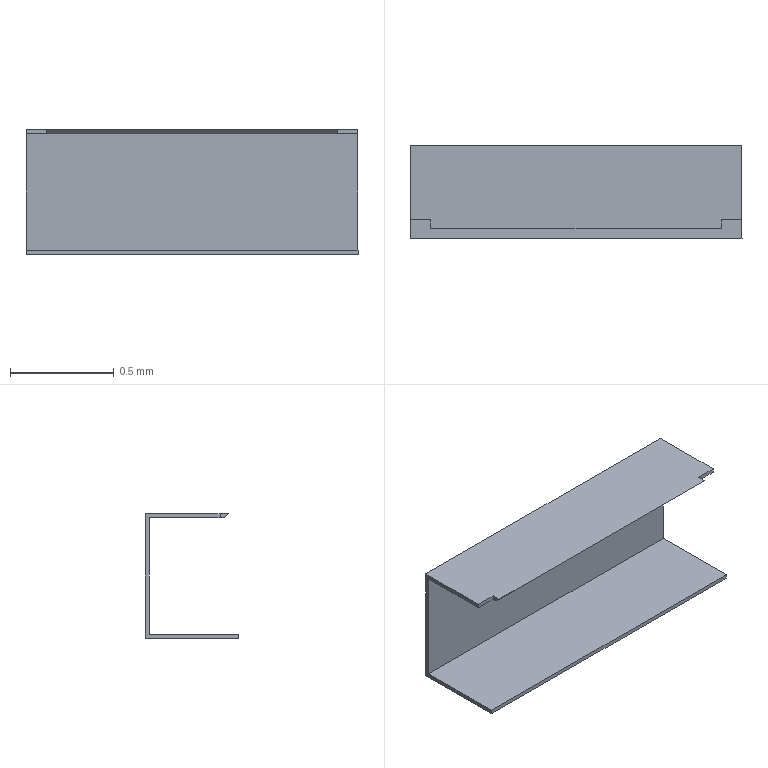Part | STEP file | RJ-USIO-V1_2-220411_11 | 1 solid | 14 faces | box 1.6 x 0.45 x 0.6 mm | volume 0.04468 mm3 | plane 14
STEP:
#1=CARTESIAN_POINT('',(0.,0.,0.));
#2=DIRECTION('',(0.,0.,1.));
#3=DIRECTION('',(1.,0.,0.));
#4=AXIS2_PLACEMENT_3D('',#1,#2,#3);
#5=CARTESIAN_POINT('',(52.5,20.72,0.58));
#6=VERTEX_POINT('',#5);
#7=CARTESIAN_POINT('',(52.5,20.74,0.58));
#8=VERTEX_POINT('',#7);
#9=CARTESIAN_POINT('',(52.5,20.72,0.58));
#10=DIRECTION('',(-0.000000044,1.,0.));
#11=VECTOR('',#10,1.);
#12=LINE('',#9,#11);
#13=CARTESIAN_POINT('',(52.5,20.74,-0.001));
#14=DIRECTION('',(-1.,-0.000000044,0.));
#15=DIRECTION('',(-0.000000044,1.,0.));
#16=AXIS2_PLACEMENT_3D('',#13,#14,#15);
#17=PLANE('',#16);
#18=CARTESIAN_POINT('',(-0.02,-0.581));
#19=DIRECTION('',(1.,0.));
#20=VECTOR('',#19,1.);
#21=LINE('',#18,#20);
#22=(GEOMETRIC_REPRESENTATION_CONTEXT(2)PARAMETRIC_REPRESENTATION_CONTEXT()REPRESENTATION_CONTEXT('',''));
#23=DEFINITIONAL_REPRESENTATION('',(#21),#22);
#24=PCURVE('',#17,#23);
#25=CARTESIAN_POINT('',(52.6,20.72,0.58));
#26=DIRECTION('',(0.,0.,-1.));
#27=DIRECTION('',(-0.000000044,1.,0.));
#28=AXIS2_PLACEMENT_3D('',#25,#26,#27);
#29=PLANE('',#28);
#30=CARTESIAN_POINT('',(0.,-0.1));
#31=DIRECTION('',(1.,0.));
#32=VECTOR('',#31,1.);
#33=LINE('',#30,#32);
#34=(GEOMETRIC_REPRESENTATION_CONTEXT(2)PARAMETRIC_REPRESENTATION_CONTEXT()REPRESENTATION_CONTEXT('',''));
#35=DEFINITIONAL_REPRESENTATION('',(#33),#34);
#36=PCURVE('',#29,#35);
#37=SURFACE_CURVE('',#12,(#24,#36),.PCURVE_S1.);
#38=EDGE_CURVE('',#6,#8,#37,.T.);
#39=ORIENTED_EDGE('',*,*,#38,.F.);
#40=CARTESIAN_POINT('',(52.5,20.7,0.6));
#41=VERTEX_POINT('',#40);
#42=CARTESIAN_POINT('',(52.5,20.7,0.6));
#43=DIRECTION('',(-0.000000031,0.7071,-0.7071));
#44=VECTOR('',#43,1.);
#45=LINE('',#42,#44);
#46=CARTESIAN_POINT('',(-0.04,-0.601));
#47=DIRECTION('',(0.7071,0.7071));
#48=VECTOR('',#47,1.);
#49=LINE('',#46,#48);
#50=(GEOMETRIC_REPRESENTATION_CONTEXT(2)PARAMETRIC_REPRESENTATION_CONTEXT()REPRESENTATION_CONTEXT('',''));
#51=DEFINITIONAL_REPRESENTATION('',(#49),#50);
#52=PCURVE('',#17,#51);
#53=CARTESIAN_POINT('',(52.6,20.7,0.6));
#54=DIRECTION('',(0.000000031,-0.7071,-0.7071));
#55=DIRECTION('',(-0.000000031,0.7071,-0.7071));
#56=AXIS2_PLACEMENT_3D('',#53,#54,#55);
#57=PLANE('',#56);
#58=CARTESIAN_POINT('',(0.,-0.1));
#59=DIRECTION('',(1.,0.));
#60=VECTOR('',#59,1.);
#61=LINE('',#58,#60);
#62=(GEOMETRIC_REPRESENTATION_CONTEXT(2)PARAMETRIC_REPRESENTATION_CONTEXT()REPRESENTATION_CONTEXT('',''));
#63=DEFINITIONAL_REPRESENTATION('',(#61),#62);
#64=PCURVE('',#57,#63);
#65=SURFACE_CURVE('',#45,(#52,#64),.PCURVE_S1.);
#66=EDGE_CURVE('',#41,#6,#65,.T.);
#67=ORIENTED_EDGE('',*,*,#66,.F.);
#68=CARTESIAN_POINT('',(52.5,20.74,0.6));
#69=VERTEX_POINT('',#68);
#70=CARTESIAN_POINT('',(52.5,20.7,0.6));
#71=DIRECTION('',(-0.000000044,1.,0.));
#72=VECTOR('',#71,1.);
#73=LINE('',#70,#72);
#74=CARTESIAN_POINT('',(-0.04,-0.601));
#75=DIRECTION('',(1.,0.));
#76=VECTOR('',#75,1.);
#77=LINE('',#74,#76);
#78=(GEOMETRIC_REPRESENTATION_CONTEXT(2)PARAMETRIC_REPRESENTATION_CONTEXT()REPRESENTATION_CONTEXT('',''));
#79=DEFINITIONAL_REPRESENTATION('',(#77),#78);
#80=PCURVE('',#17,#79);
#81=CARTESIAN_POINT('',(52.6,21.1,0.6));
#82=DIRECTION('',(0.,0.,1.));
#83=DIRECTION('',(0.000000044,-1.,0.));
#84=AXIS2_PLACEMENT_3D('',#81,#82,#83);
#85=PLANE('',#84);
#86=CARTESIAN_POINT('',(0.4,-0.1));
#87=DIRECTION('',(-1.,0.));
#88=VECTOR('',#87,1.);
#89=LINE('',#86,#88);
#90=(GEOMETRIC_REPRESENTATION_CONTEXT(2)PARAMETRIC_REPRESENTATION_CONTEXT()REPRESENTATION_CONTEXT('',''));
#91=DEFINITIONAL_REPRESENTATION('',(#89),#90);
#92=PCURVE('',#85,#91);
#93=SURFACE_CURVE('',#73,(#80,#92),.PCURVE_S1.);
#94=EDGE_CURVE('',#41,#69,#93,.T.);
#95=ORIENTED_EDGE('',*,*,#94,.T.);
#96=CARTESIAN_POINT('',(52.5,20.74,0.6));
#97=DIRECTION('',(0.,0.,-1.));
#98=VECTOR('',#97,1.);
#99=LINE('',#96,#98);
#100=CARTESIAN_POINT('',(0.,-0.601));
#101=DIRECTION('',(0.,1.));
#102=VECTOR('',#101,1.);
#103=LINE('',#100,#102);
#104=(GEOMETRIC_REPRESENTATION_CONTEXT(2)PARAMETRIC_REPRESENTATION_CONTEXT()REPRESENTATION_CONTEXT('',''));
#105=DEFINITIONAL_REPRESENTATION('',(#103),#104);
#106=PCURVE('',#17,#105);
#107=CARTESIAN_POINT('',(52.6,20.74,-0.001));
#108=DIRECTION('',(-0.000000044,1.,0.));
#109=DIRECTION('',(0.,0.,1.));
#110=AXIS2_PLACEMENT_3D('',#107,#108,#109);
#111=PLANE('',#110);
#112=CARTESIAN_POINT('',(0.601,-0.1));
#113=DIRECTION('',(-1.,0.));
#114=VECTOR('',#113,1.);
#115=LINE('',#112,#114);
#116=(GEOMETRIC_REPRESENTATION_CONTEXT(2)PARAMETRIC_REPRESENTATION_CONTEXT()REPRESENTATION_CONTEXT('',''));
#117=DEFINITIONAL_REPRESENTATION('',(#115),#116);
#118=PCURVE('',#111,#117);
#119=SURFACE_CURVE('',#99,(#106,#118),.PCURVE_S1.);
#120=EDGE_CURVE('',#69,#8,#119,.T.);
#121=ORIENTED_EDGE('',*,*,#120,.T.);
#122=EDGE_LOOP('',(#39,#67,#95,#121));
#123=FACE_BOUND('',#122,.F.);
#124=ADVANCED_FACE('',(#123),#17,.F.);
#125=CARTESIAN_POINT('',(51.1,20.74,0.58));
#126=VERTEX_POINT('',#125);
#127=CARTESIAN_POINT('',(51.1,20.72,0.58));
#128=VERTEX_POINT('',#127);
#129=CARTESIAN_POINT('',(51.1,20.74,0.58));
#130=DIRECTION('',(0.000000044,-1.,0.));
#131=VECTOR('',#130,1.);
#132=LINE('',#129,#131);
#133=CARTESIAN_POINT('',(0.02,-1.5));
#134=DIRECTION('',(-1.,0.));
#135=VECTOR('',#134,1.);
#136=LINE('',#133,#135);
#137=(GEOMETRIC_REPRESENTATION_CONTEXT(2)PARAMETRIC_REPRESENTATION_CONTEXT()REPRESENTATION_CONTEXT('',''));
#138=DEFINITIONAL_REPRESENTATION('',(#136),#137);
#139=PCURVE('',#29,#138);
#140=CARTESIAN_POINT('',(51.1,20.74,-0.001));
#141=DIRECTION('',(1.,0.000000044,0.));
#142=DIRECTION('',(0.000000044,-1.,0.));
#143=AXIS2_PLACEMENT_3D('',#140,#141,#142);
#144=PLANE('',#143);
#145=CARTESIAN_POINT('',(0.,-0.581));
#146=DIRECTION('',(1.,0.));
#147=VECTOR('',#146,1.);
#148=LINE('',#145,#147);
#149=(GEOMETRIC_REPRESENTATION_CONTEXT(2)PARAMETRIC_REPRESENTATION_CONTEXT()REPRESENTATION_CONTEXT('',''));
#150=DEFINITIONAL_REPRESENTATION('',(#148),#149);
#151=PCURVE('',#144,#150);
#152=SURFACE_CURVE('',#132,(#139,#151),.PCURVE_S1.);
#153=EDGE_CURVE('',#126,#128,#152,.T.);
#154=ORIENTED_EDGE('',*,*,#153,.T.);
#155=CARTESIAN_POINT('',(51.1,20.72,0.58));
#156=DIRECTION('',(1.,0.000000044,0.));
#157=VECTOR('',#156,1.);
#158=LINE('',#155,#157);
#159=CARTESIAN_POINT('',(0.,-1.5));
#160=DIRECTION('',(0.,1.));
#161=VECTOR('',#160,1.);
#162=LINE('',#159,#161);
#163=(GEOMETRIC_REPRESENTATION_CONTEXT(2)PARAMETRIC_REPRESENTATION_CONTEXT()REPRESENTATION_CONTEXT('',''));
#164=DEFINITIONAL_REPRESENTATION('',(#162),#163);
#165=PCURVE('',#29,#164);
#166=CARTESIAN_POINT('',(0.02828,-1.5));
#167=DIRECTION('',(0.,1.));
#168=VECTOR('',#167,1.);
#169=LINE('',#166,#168);
#170=(GEOMETRIC_REPRESENTATION_CONTEXT(2)PARAMETRIC_REPRESENTATION_CONTEXT()REPRESENTATION_CONTEXT('',''));
#171=DEFINITIONAL_REPRESENTATION('',(#169),#170);
#172=PCURVE('',#57,#171);
#173=SURFACE_CURVE('',#158,(#165,#172),.PCURVE_S1.);
#174=EDGE_CURVE('',#128,#6,#173,.T.);
#175=ORIENTED_EDGE('',*,*,#174,.T.);
#176=ORIENTED_EDGE('',*,*,#38,.T.);
#177=CARTESIAN_POINT('',(52.6,20.74,0.58));
#178=VERTEX_POINT('',#177);
#179=CARTESIAN_POINT('',(52.5,20.74,0.58));
#180=DIRECTION('',(1.,0.000000044,0.));
#181=VECTOR('',#180,1.);
#182=LINE('',#179,#181);
#183=CARTESIAN_POINT('',(0.02,-0.1));
#184=DIRECTION('',(0.,1.));
#185=VECTOR('',#184,1.);
#186=LINE('',#183,#185);
#187=(GEOMETRIC_REPRESENTATION_CONTEXT(2)PARAMETRIC_REPRESENTATION_CONTEXT()REPRESENTATION_CONTEXT('',''));
#188=DEFINITIONAL_REPRESENTATION('',(#186),#187);
#189=PCURVE('',#29,#188);
#190=CARTESIAN_POINT('',(0.581,-0.1));
#191=DIRECTION('',(0.,1.));
#192=VECTOR('',#191,1.);
#193=LINE('',#190,#192);
#194=(GEOMETRIC_REPRESENTATION_CONTEXT(2)PARAMETRIC_REPRESENTATION_CONTEXT()REPRESENTATION_CONTEXT('',''));
#195=DEFINITIONAL_REPRESENTATION('',(#193),#194);
#196=PCURVE('',#111,#195);
#197=SURFACE_CURVE('',#182,(#189,#196),.PCURVE_S1.);
#198=EDGE_CURVE('',#8,#178,#197,.T.);
#199=ORIENTED_EDGE('',*,*,#198,.T.);
#200=CARTESIAN_POINT('',(52.6,21.08,0.58));
#201=VERTEX_POINT('',#200);
#202=CARTESIAN_POINT('',(52.6,20.74,0.58));
#203=DIRECTION('',(-0.000000044,1.,0.));
#204=VECTOR('',#203,1.);
#205=LINE('',#202,#204);
#206=CARTESIAN_POINT('',(0.02,0.));
#207=DIRECTION('',(1.,0.));
#208=VECTOR('',#207,1.);
#209=LINE('',#206,#208);
#210=(GEOMETRIC_REPRESENTATION_CONTEXT(2)PARAMETRIC_REPRESENTATION_CONTEXT()REPRESENTATION_CONTEXT('',''));
#211=DEFINITIONAL_REPRESENTATION('',(#209),#210);
#212=PCURVE('',#29,#211);
#213=CARTESIAN_POINT('',(52.6,19.5,0.));
#214=DIRECTION('',(1.,0.000000044,0.));
#215=DIRECTION('',(0.,0.,1.));
#216=AXIS2_PLACEMENT_3D('',#213,#214,#215);
#217=PLANE('',#216);
#218=CARTESIAN_POINT('',(0.58,-1.24));
#219=DIRECTION('',(0.,-1.));
#220=VECTOR('',#219,1.);
#221=LINE('',#218,#220);
#222=(GEOMETRIC_REPRESENTATION_CONTEXT(2)PARAMETRIC_REPRESENTATION_CONTEXT()REPRESENTATION_CONTEXT('',''));
#223=DEFINITIONAL_REPRESENTATION('',(#221),#222);
#224=PCURVE('',#217,#223);
#225=SURFACE_CURVE('',#205,(#212,#224),.PCURVE_S1.);
#226=EDGE_CURVE('',#178,#201,#225,.T.);
#227=ORIENTED_EDGE('',*,*,#226,.T.);
#228=CARTESIAN_POINT('',(51.,21.08,0.58));
#229=VERTEX_POINT('',#228);
#230=CARTESIAN_POINT('',(51.,21.08,0.58));
#231=DIRECTION('',(1.,0.000000044,0.));
#232=VECTOR('',#231,1.);
#233=LINE('',#230,#232);
#234=CARTESIAN_POINT('',(0.36,-1.6));
#235=DIRECTION('',(0.,1.));
#236=VECTOR('',#235,1.);
#237=LINE('',#234,#236);
#238=(GEOMETRIC_REPRESENTATION_CONTEXT(2)PARAMETRIC_REPRESENTATION_CONTEXT()REPRESENTATION_CONTEXT('',''));
#239=DEFINITIONAL_REPRESENTATION('',(#237),#238);
#240=PCURVE('',#29,#239);
#241=CARTESIAN_POINT('',(52.6,21.08,0.58));
#242=DIRECTION('',(0.000000044,-1.,0.));
#243=DIRECTION('',(0.,0.,-1.));
#244=AXIS2_PLACEMENT_3D('',#241,#242,#243);
#245=PLANE('',#244);
#246=CARTESIAN_POINT('',(0.,-1.6));
#247=DIRECTION('',(0.,1.));
#248=VECTOR('',#247,1.);
#249=LINE('',#246,#248);
#250=(GEOMETRIC_REPRESENTATION_CONTEXT(2)PARAMETRIC_REPRESENTATION_CONTEXT()REPRESENTATION_CONTEXT('',''));
#251=DEFINITIONAL_REPRESENTATION('',(#249),#250);
#252=PCURVE('',#245,#251);
#253=SURFACE_CURVE('',#233,(#240,#252),.PCURVE_S1.);
#254=EDGE_CURVE('',#229,#201,#253,.T.);
#255=ORIENTED_EDGE('',*,*,#254,.F.);
#256=CARTESIAN_POINT('',(51.,20.74,0.58));
#257=VERTEX_POINT('',#256);
#258=CARTESIAN_POINT('',(51.,20.74,0.58));
#259=DIRECTION('',(-0.000000044,1.,0.));
#260=VECTOR('',#259,1.);
#261=LINE('',#258,#260);
#262=CARTESIAN_POINT('',(0.02,-1.6));
#263=DIRECTION('',(1.,0.));
#264=VECTOR('',#263,1.);
#265=LINE('',#262,#264);
#266=(GEOMETRIC_REPRESENTATION_CONTEXT(2)PARAMETRIC_REPRESENTATION_CONTEXT()REPRESENTATION_CONTEXT('',''));
#267=DEFINITIONAL_REPRESENTATION('',(#265),#266);
#268=PCURVE('',#29,#267);
#269=CARTESIAN_POINT('',(51.,19.5,0.));
#270=DIRECTION('',(1.,0.000000044,0.));
#271=DIRECTION('',(0.,0.,1.));
#272=AXIS2_PLACEMENT_3D('',#269,#270,#271);
#273=PLANE('',#272);
#274=CARTESIAN_POINT('',(0.58,-1.24));
#275=DIRECTION('',(0.,-1.));
#276=VECTOR('',#275,1.);
#277=LINE('',#274,#276);
#278=(GEOMETRIC_REPRESENTATION_CONTEXT(2)PARAMETRIC_REPRESENTATION_CONTEXT()REPRESENTATION_CONTEXT('',''));
#279=DEFINITIONAL_REPRESENTATION('',(#277),#278);
#280=PCURVE('',#273,#279);
#281=SURFACE_CURVE('',#261,(#268,#280),.PCURVE_S1.);
#282=EDGE_CURVE('',#257,#229,#281,.T.);
#283=ORIENTED_EDGE('',*,*,#282,.F.);
#284=CARTESIAN_POINT('',(51.,20.74,0.58));
#285=DIRECTION('',(1.,0.000000044,0.));
#286=VECTOR('',#285,1.);
#287=LINE('',#284,#286);
#288=CARTESIAN_POINT('',(0.02,-1.6));
#289=DIRECTION('',(0.,1.));
#290=VECTOR('',#289,1.);
#291=LINE('',#288,#290);
#292=(GEOMETRIC_REPRESENTATION_CONTEXT(2)PARAMETRIC_REPRESENTATION_CONTEXT()REPRESENTATION_CONTEXT('',''));
#293=DEFINITIONAL_REPRESENTATION('',(#291),#292);
#294=PCURVE('',#29,#293);
#295=CARTESIAN_POINT('',(51.,20.74,-0.001));
#296=DIRECTION('',(-0.000000044,1.,0.));
#297=DIRECTION('',(0.,0.,1.));
#298=AXIS2_PLACEMENT_3D('',#295,#296,#297);
#299=PLANE('',#298);
#300=CARTESIAN_POINT('',(0.581,0.));
#301=DIRECTION('',(0.,1.));
#302=VECTOR('',#301,1.);
#303=LINE('',#300,#302);
#304=(GEOMETRIC_REPRESENTATION_CONTEXT(2)PARAMETRIC_REPRESENTATION_CONTEXT()REPRESENTATION_CONTEXT('',''));
#305=DEFINITIONAL_REPRESENTATION('',(#303),#304);
#306=PCURVE('',#299,#305);
#307=SURFACE_CURVE('',#287,(#294,#306),.PCURVE_S1.);
#308=EDGE_CURVE('',#257,#126,#307,.T.);
#309=ORIENTED_EDGE('',*,*,#308,.T.);
#310=EDGE_LOOP('',(#154,#175,#176,#199,#227,#255,#283,#309));
#311=FACE_BOUND('',#310,.F.);
#312=ADVANCED_FACE('',(#311),#29,.T.);
#313=CARTESIAN_POINT('',(51.1,20.74,0.6));
#314=VERTEX_POINT('',#313);
#315=CARTESIAN_POINT('',(51.1,20.7,0.6));
#316=VERTEX_POINT('',#315);
#317=CARTESIAN_POINT('',(51.1,20.74,0.6));
#318=DIRECTION('',(0.000000044,-1.,0.));
#319=VECTOR('',#318,1.);
#320=LINE('',#317,#319);
#321=CARTESIAN_POINT('',(0.,-0.601));
#322=DIRECTION('',(1.,0.));
#323=VECTOR('',#322,1.);
#324=LINE('',#321,#323);
#325=(GEOMETRIC_REPRESENTATION_CONTEXT(2)PARAMETRIC_REPRESENTATION_CONTEXT()REPRESENTATION_CONTEXT('',''));
#326=DEFINITIONAL_REPRESENTATION('',(#324),#325);
#327=PCURVE('',#144,#326);
#328=CARTESIAN_POINT('',(0.36,-1.5));
#329=DIRECTION('',(1.,0.));
#330=VECTOR('',#329,1.);
#331=LINE('',#328,#330);
#332=(GEOMETRIC_REPRESENTATION_CONTEXT(2)PARAMETRIC_REPRESENTATION_CONTEXT()REPRESENTATION_CONTEXT('',''));
#333=DEFINITIONAL_REPRESENTATION('',(#331),#332);
#334=PCURVE('',#85,#333);
#335=SURFACE_CURVE('',#320,(#327,#334),.PCURVE_S1.);
#336=EDGE_CURVE('',#314,#316,#335,.T.);
#337=ORIENTED_EDGE('',*,*,#336,.T.);
#338=CARTESIAN_POINT('',(51.1,20.72,0.58));
#339=DIRECTION('',(0.000000031,-0.7071,0.7071));
#340=VECTOR('',#339,1.);
#341=LINE('',#338,#340);
#342=CARTESIAN_POINT('',(0.02,-0.581));
#343=DIRECTION('',(0.7071,-0.7071));
#344=VECTOR('',#343,1.);
#345=LINE('',#342,#344);
#346=(GEOMETRIC_REPRESENTATION_CONTEXT(2)PARAMETRIC_REPRESENTATION_CONTEXT()REPRESENTATION_CONTEXT('',''));
#347=DEFINITIONAL_REPRESENTATION('',(#345),#346);
#348=PCURVE('',#144,#347);
#349=CARTESIAN_POINT('',(0.02828,-1.5));
#350=DIRECTION('',(-1.,0.));
#351=VECTOR('',#350,1.);
#352=LINE('',#349,#351);
#353=(GEOMETRIC_REPRESENTATION_CONTEXT(2)PARAMETRIC_REPRESENTATION_CONTEXT()REPRESENTATION_CONTEXT('',''));
#354=DEFINITIONAL_REPRESENTATION('',(#352),#353);
#355=PCURVE('',#57,#354);
#356=SURFACE_CURVE('',#341,(#348,#355),.PCURVE_S1.);
#357=EDGE_CURVE('',#128,#316,#356,.T.);
#358=ORIENTED_EDGE('',*,*,#357,.F.);
#359=ORIENTED_EDGE('',*,*,#153,.F.);
#360=CARTESIAN_POINT('',(51.1,20.74,0.6));
#361=DIRECTION('',(0.,0.,-1.));
#362=VECTOR('',#361,1.);
#363=LINE('',#360,#362);
#364=CARTESIAN_POINT('',(0.,-0.601));
#365=DIRECTION('',(0.,1.));
#366=VECTOR('',#365,1.);
#367=LINE('',#364,#366);
#368=(GEOMETRIC_REPRESENTATION_CONTEXT(2)PARAMETRIC_REPRESENTATION_CONTEXT()REPRESENTATION_CONTEXT('',''));
#369=DEFINITIONAL_REPRESENTATION('',(#367),#368);
#370=PCURVE('',#144,#369);
#371=CARTESIAN_POINT('',(0.601,0.1));
#372=DIRECTION('',(-1.,0.));
#373=VECTOR('',#372,1.);
#374=LINE('',#371,#373);
#375=(GEOMETRIC_REPRESENTATION_CONTEXT(2)PARAMETRIC_REPRESENTATION_CONTEXT()REPRESENTATION_CONTEXT('',''));
#376=DEFINITIONAL_REPRESENTATION('',(#374),#375);
#377=PCURVE('',#299,#376);
#378=SURFACE_CURVE('',#363,(#370,#377),.PCURVE_S1.);
#379=EDGE_CURVE('',#314,#126,#378,.T.);
#380=ORIENTED_EDGE('',*,*,#379,.F.);
#381=EDGE_LOOP('',(#337,#358,#359,#380));
#382=FACE_BOUND('',#381,.F.);
#383=ADVANCED_FACE('',(#382),#144,.F.);
#384=ORIENTED_EDGE('',*,*,#336,.F.);
#385=CARTESIAN_POINT('',(51.,20.74,0.6));
#386=VERTEX_POINT('',#385);
#387=CARTESIAN_POINT('',(51.,20.74,0.6));
#388=DIRECTION('',(1.,0.000000044,0.));
#389=VECTOR('',#388,1.);
#390=LINE('',#387,#389);
#391=CARTESIAN_POINT('',(0.36,-1.6));
#392=DIRECTION('',(0.,1.));
#393=VECTOR('',#392,1.);
#394=LINE('',#391,#393);
#395=(GEOMETRIC_REPRESENTATION_CONTEXT(2)PARAMETRIC_REPRESENTATION_CONTEXT()REPRESENTATION_CONTEXT('',''));
#396=DEFINITIONAL_REPRESENTATION('',(#394),#395);
#397=PCURVE('',#85,#396);
#398=CARTESIAN_POINT('',(0.601,0.));
#399=DIRECTION('',(0.,1.));
#400=VECTOR('',#399,1.);
#401=LINE('',#398,#400);
#402=(GEOMETRIC_REPRESENTATION_CONTEXT(2)PARAMETRIC_REPRESENTATION_CONTEXT()REPRESENTATION_CONTEXT('',''));
#403=DEFINITIONAL_REPRESENTATION('',(#401),#402);
#404=PCURVE('',#299,#403);
#405=SURFACE_CURVE('',#390,(#397,#404),.PCURVE_S1.);
#406=EDGE_CURVE('',#386,#314,#405,.T.);
#407=ORIENTED_EDGE('',*,*,#406,.F.);
#408=CARTESIAN_POINT('',(51.,21.1,0.6));
#409=VERTEX_POINT('',#408);
#410=CARTESIAN_POINT('',(51.,21.1,0.6));
#411=DIRECTION('',(0.000000044,-1.,0.));
#412=VECTOR('',#411,1.);
#413=LINE('',#410,#412);
#414=CARTESIAN_POINT('',(0.,-1.6));
#415=DIRECTION('',(1.,0.));
#416=VECTOR('',#415,1.);
#417=LINE('',#414,#416);
#418=(GEOMETRIC_REPRESENTATION_CONTEXT(2)PARAMETRIC_REPRESENTATION_CONTEXT()REPRESENTATION_CONTEXT('',''));
#419=DEFINITIONAL_REPRESENTATION('',(#417),#418);
#420=PCURVE('',#85,#419);
#421=CARTESIAN_POINT('',(0.6,-1.6));
#422=DIRECTION('',(0.,1.));
#423=VECTOR('',#422,1.);
#424=LINE('',#421,#423);
#425=(GEOMETRIC_REPRESENTATION_CONTEXT(2)PARAMETRIC_REPRESENTATION_CONTEXT()REPRESENTATION_CONTEXT('',''));
#426=DEFINITIONAL_REPRESENTATION('',(#424),#425);
#427=PCURVE('',#273,#426);
#428=SURFACE_CURVE('',#413,(#420,#427),.PCURVE_S1.);
#429=EDGE_CURVE('',#409,#386,#428,.T.);
#430=ORIENTED_EDGE('',*,*,#429,.F.);
#431=CARTESIAN_POINT('',(52.6,21.1,0.6));
#432=VERTEX_POINT('',#431);
#433=CARTESIAN_POINT('',(51.,21.1,0.6));
#434=DIRECTION('',(1.,0.000000044,0.));
#435=VECTOR('',#434,1.);
#436=LINE('',#433,#435);
#437=CARTESIAN_POINT('',(0.,-1.6));
#438=DIRECTION('',(0.,1.));
#439=VECTOR('',#438,1.);
#440=LINE('',#437,#439);
#441=(GEOMETRIC_REPRESENTATION_CONTEXT(2)PARAMETRIC_REPRESENTATION_CONTEXT()REPRESENTATION_CONTEXT('',''));
#442=DEFINITIONAL_REPRESENTATION('',(#440),#441);
#443=PCURVE('',#85,#442);
#444=CARTESIAN_POINT('',(52.6,21.1,0.));
#445=DIRECTION('',(-0.000000044,1.,0.));
#446=DIRECTION('',(0.,0.,1.));
#447=AXIS2_PLACEMENT_3D('',#444,#445,#446);
#448=PLANE('',#447);
#449=CARTESIAN_POINT('',(0.6,-1.6));
#450=DIRECTION('',(0.,1.));
#451=VECTOR('',#450,1.);
#452=LINE('',#449,#451);
#453=(GEOMETRIC_REPRESENTATION_CONTEXT(2)PARAMETRIC_REPRESENTATION_CONTEXT()REPRESENTATION_CONTEXT('',''));
#454=DEFINITIONAL_REPRESENTATION('',(#452),#453);
#455=PCURVE('',#448,#454);
#456=SURFACE_CURVE('',#436,(#443,#455),.PCURVE_S1.);
#457=EDGE_CURVE('',#409,#432,#456,.T.);
#458=ORIENTED_EDGE('',*,*,#457,.T.);
#459=CARTESIAN_POINT('',(52.6,20.74,0.6));
#460=VERTEX_POINT('',#459);
#461=CARTESIAN_POINT('',(52.6,21.1,0.6));
#462=DIRECTION('',(0.000000044,-1.,0.));
#463=VECTOR('',#462,1.);
#464=LINE('',#461,#463);
#465=CARTESIAN_POINT('',(0.,0.));
#466=DIRECTION('',(1.,0.));
#467=VECTOR('',#466,1.);
#468=LINE('',#465,#467);
#469=(GEOMETRIC_REPRESENTATION_CONTEXT(2)PARAMETRIC_REPRESENTATION_CONTEXT()REPRESENTATION_CONTEXT('',''));
#470=DEFINITIONAL_REPRESENTATION('',(#468),#469);
#471=PCURVE('',#85,#470);
#472=CARTESIAN_POINT('',(0.6,-1.6));
#473=DIRECTION('',(0.,1.));
#474=VECTOR('',#473,1.);
#475=LINE('',#472,#474);
#476=(GEOMETRIC_REPRESENTATION_CONTEXT(2)PARAMETRIC_REPRESENTATION_CONTEXT()REPRESENTATION_CONTEXT('',''));
#477=DEFINITIONAL_REPRESENTATION('',(#475),#476);
#478=PCURVE('',#217,#477);
#479=SURFACE_CURVE('',#464,(#471,#478),.PCURVE_S1.);
#480=EDGE_CURVE('',#432,#460,#479,.T.);
#481=ORIENTED_EDGE('',*,*,#480,.T.);
#482=CARTESIAN_POINT('',(52.5,20.74,0.6));
#483=DIRECTION('',(1.,0.000000044,0.));
#484=VECTOR('',#483,1.);
#485=LINE('',#482,#484);
#486=CARTESIAN_POINT('',(0.36,-0.1));
#487=DIRECTION('',(0.,1.));
#488=VECTOR('',#487,1.);
#489=LINE('',#486,#488);
#490=(GEOMETRIC_REPRESENTATION_CONTEXT(2)PARAMETRIC_REPRESENTATION_CONTEXT()REPRESENTATION_CONTEXT('',''));
#491=DEFINITIONAL_REPRESENTATION('',(#489),#490);
#492=PCURVE('',#85,#491);
#493=CARTESIAN_POINT('',(0.601,-0.1));
#494=DIRECTION('',(0.,1.));
#495=VECTOR('',#494,1.);
#496=LINE('',#493,#495);
#497=(GEOMETRIC_REPRESENTATION_CONTEXT(2)PARAMETRIC_REPRESENTATION_CONTEXT()REPRESENTATION_CONTEXT('',''));
#498=DEFINITIONAL_REPRESENTATION('',(#496),#497);
#499=PCURVE('',#111,#498);
#500=SURFACE_CURVE('',#485,(#492,#499),.PCURVE_S1.);
#501=EDGE_CURVE('',#69,#460,#500,.T.);
#502=ORIENTED_EDGE('',*,*,#501,.F.);
#503=ORIENTED_EDGE('',*,*,#94,.F.);
#504=CARTESIAN_POINT('',(51.1,20.7,0.6));
#505=DIRECTION('',(1.,0.000000044,0.));
#506=VECTOR('',#505,1.);
#507=LINE('',#504,#506);
#508=CARTESIAN_POINT('',(0.4,-1.5));
#509=DIRECTION('',(0.,1.));
#510=VECTOR('',#509,1.);
#511=LINE('',#508,#510);
#512=(GEOMETRIC_REPRESENTATION_CONTEXT(2)PARAMETRIC_REPRESENTATION_CONTEXT()REPRESENTATION_CONTEXT('',''));
#513=DEFINITIONAL_REPRESENTATION('',(#511),#512);
#514=PCURVE('',#85,#513);
#515=CARTESIAN_POINT('',(0.,-1.5));
#516=DIRECTION('',(0.,1.));
#517=VECTOR('',#516,1.);
#518=LINE('',#515,#517);
#519=(GEOMETRIC_REPRESENTATION_CONTEXT(2)PARAMETRIC_REPRESENTATION_CONTEXT()REPRESENTATION_CONTEXT('',''));
#520=DEFINITIONAL_REPRESENTATION('',(#518),#519);
#521=PCURVE('',#57,#520);
#522=SURFACE_CURVE('',#507,(#514,#521),.PCURVE_S1.);
#523=EDGE_CURVE('',#316,#41,#522,.T.);
#524=ORIENTED_EDGE('',*,*,#523,.F.);
#525=EDGE_LOOP('',(#384,#407,#430,#458,#481,#502,#503,#524));
#526=FACE_BOUND('',#525,.F.);
#527=ADVANCED_FACE('',(#526),#85,.T.);
#528=ORIENTED_EDGE('',*,*,#379,.T.);
#529=ORIENTED_EDGE('',*,*,#308,.F.);
#530=CARTESIAN_POINT('',(51.,20.74,0.6));
#531=DIRECTION('',(0.,0.,-1.));
#532=VECTOR('',#531,1.);
#533=LINE('',#530,#532);
#534=CARTESIAN_POINT('',(0.601,0.));
#535=DIRECTION('',(-1.,0.));
#536=VECTOR('',#535,1.);
#537=LINE('',#534,#536);
#538=(GEOMETRIC_REPRESENTATION_CONTEXT(2)PARAMETRIC_REPRESENTATION_CONTEXT()REPRESENTATION_CONTEXT('',''));
#539=DEFINITIONAL_REPRESENTATION('',(#537),#538);
#540=PCURVE('',#299,#539);
#541=CARTESIAN_POINT('',(0.6,-1.24));
#542=DIRECTION('',(-1.,0.));
#543=VECTOR('',#542,1.);
#544=LINE('',#541,#543);
#545=(GEOMETRIC_REPRESENTATION_CONTEXT(2)PARAMETRIC_REPRESENTATION_CONTEXT()REPRESENTATION_CONTEXT('',''));
#546=DEFINITIONAL_REPRESENTATION('',(#544),#545);
#547=PCURVE('',#273,#546);
#548=SURFACE_CURVE('',#533,(#540,#547),.PCURVE_S1.);
#549=EDGE_CURVE('',#386,#257,#548,.T.);
#550=ORIENTED_EDGE('',*,*,#549,.F.);
#551=ORIENTED_EDGE('',*,*,#406,.T.);
#552=EDGE_LOOP('',(#528,#529,#550,#551));
#553=FACE_BOUND('',#552,.F.);
#554=ADVANCED_FACE('',(#553),#299,.F.);
#555=ORIENTED_EDGE('',*,*,#282,.T.);
#556=CARTESIAN_POINT('',(51.,21.08,0.02));
#557=VERTEX_POINT('',#556);
#558=CARTESIAN_POINT('',(51.,21.08,0.58));
#559=DIRECTION('',(0.,0.,-1.));
#560=VECTOR('',#559,1.);
#561=LINE('',#558,#560);
#562=CARTESIAN_POINT('',(0.58,-1.58));
#563=DIRECTION('',(-1.,0.));
#564=VECTOR('',#563,1.);
#565=LINE('',#562,#564);
#566=(GEOMETRIC_REPRESENTATION_CONTEXT(2)PARAMETRIC_REPRESENTATION_CONTEXT()REPRESENTATION_CONTEXT('',''));
#567=DEFINITIONAL_REPRESENTATION('',(#565),#566);
#568=PCURVE('',#273,#567);
#569=CARTESIAN_POINT('',(0.,-1.6));
#570=DIRECTION('',(1.,0.));
#571=VECTOR('',#570,1.);
#572=LINE('',#569,#571);
#573=(GEOMETRIC_REPRESENTATION_CONTEXT(2)PARAMETRIC_REPRESENTATION_CONTEXT()REPRESENTATION_CONTEXT('',''));
#574=DEFINITIONAL_REPRESENTATION('',(#572),#573);
#575=PCURVE('',#245,#574);
#576=SURFACE_CURVE('',#561,(#568,#575),.PCURVE_S1.);
#577=EDGE_CURVE('',#229,#557,#576,.T.);
#578=ORIENTED_EDGE('',*,*,#577,.T.);
#579=CARTESIAN_POINT('',(51.,20.65,0.02));
#580=VERTEX_POINT('',#579);
#581=CARTESIAN_POINT('',(51.,21.08,0.02));
#582=DIRECTION('',(0.000000044,-1.,0.));
#583=VECTOR('',#582,1.);
#584=LINE('',#581,#583);
#585=CARTESIAN_POINT('',(0.02,-1.58));
#586=DIRECTION('',(0.,1.));
#587=VECTOR('',#586,1.);
#588=LINE('',#585,#587);
#589=(GEOMETRIC_REPRESENTATION_CONTEXT(2)PARAMETRIC_REPRESENTATION_CONTEXT()REPRESENTATION_CONTEXT('',''));
#590=DEFINITIONAL_REPRESENTATION('',(#588),#589);
#591=PCURVE('',#273,#590);
#592=CARTESIAN_POINT('',(52.6,21.08,0.02));
#593=DIRECTION('',(0.,0.,1.));
#594=DIRECTION('',(0.000000044,-1.,0.));
#595=AXIS2_PLACEMENT_3D('',#592,#593,#594);
#596=PLANE('',#595);
#597=CARTESIAN_POINT('',(0.,-1.6));
#598=DIRECTION('',(1.,0.));
#599=VECTOR('',#598,1.);
#600=LINE('',#597,#599);
#601=(GEOMETRIC_REPRESENTATION_CONTEXT(2)PARAMETRIC_REPRESENTATION_CONTEXT()REPRESENTATION_CONTEXT('',''));
#602=DEFINITIONAL_REPRESENTATION('',(#600),#601);
#603=PCURVE('',#596,#602);
#604=SURFACE_CURVE('',#584,(#591,#603),.PCURVE_S1.);
#605=EDGE_CURVE('',#557,#580,#604,.T.);
#606=ORIENTED_EDGE('',*,*,#605,.T.);
#607=CARTESIAN_POINT('',(51.,20.65,0.));
#608=VERTEX_POINT('',#607);
#609=CARTESIAN_POINT('',(51.,20.65,0.02));
#610=DIRECTION('',(0.,0.,-1.));
#611=VECTOR('',#610,1.);
#612=LINE('',#609,#611);
#613=CARTESIAN_POINT('',(0.02,-1.15));
#614=DIRECTION('',(-1.,0.));
#615=VECTOR('',#614,1.);
#616=LINE('',#613,#615);
#617=(GEOMETRIC_REPRESENTATION_CONTEXT(2)PARAMETRIC_REPRESENTATION_CONTEXT()REPRESENTATION_CONTEXT('',''));
#618=DEFINITIONAL_REPRESENTATION('',(#616),#617);
#619=PCURVE('',#273,#618);
#620=CARTESIAN_POINT('',(52.6,20.65,0.02));
#621=DIRECTION('',(0.000000044,-1.,0.));
#622=DIRECTION('',(0.,0.,-1.));
#623=AXIS2_PLACEMENT_3D('',#620,#621,#622);
#624=PLANE('',#623);
#625=CARTESIAN_POINT('',(0.,-1.6));
#626=DIRECTION('',(1.,0.));
#627=VECTOR('',#626,1.);
#628=LINE('',#625,#627);
#629=(GEOMETRIC_REPRESENTATION_CONTEXT(2)PARAMETRIC_REPRESENTATION_CONTEXT()REPRESENTATION_CONTEXT('',''));
#630=DEFINITIONAL_REPRESENTATION('',(#628),#629);
#631=PCURVE('',#624,#630);
#632=SURFACE_CURVE('',#612,(#619,#631),.PCURVE_S1.);
#633=EDGE_CURVE('',#580,#608,#632,.T.);
#634=ORIENTED_EDGE('',*,*,#633,.T.);
#635=CARTESIAN_POINT('',(51.,21.1,0.));
#636=VERTEX_POINT('',#635);
#637=CARTESIAN_POINT('',(51.,20.65,0.));
#638=DIRECTION('',(-0.000000044,1.,0.));
#639=VECTOR('',#638,1.);
#640=LINE('',#637,#639);
#641=CARTESIAN_POINT('',(0.,-1.15));
#642=DIRECTION('',(0.,-1.));
#643=VECTOR('',#642,1.);
#644=LINE('',#641,#643);
#645=(GEOMETRIC_REPRESENTATION_CONTEXT(2)PARAMETRIC_REPRESENTATION_CONTEXT()REPRESENTATION_CONTEXT('',''));
#646=DEFINITIONAL_REPRESENTATION('',(#644),#645);
#647=PCURVE('',#273,#646);
#648=CARTESIAN_POINT('',(52.6,20.65,0.));
#649=DIRECTION('',(0.,0.,-1.));
#650=DIRECTION('',(-0.000000044,1.,0.));
#651=AXIS2_PLACEMENT_3D('',#648,#649,#650);
#652=PLANE('',#651);
#653=CARTESIAN_POINT('',(0.,-1.6));
#654=DIRECTION('',(1.,0.));
#655=VECTOR('',#654,1.);
#656=LINE('',#653,#655);
#657=(GEOMETRIC_REPRESENTATION_CONTEXT(2)PARAMETRIC_REPRESENTATION_CONTEXT()REPRESENTATION_CONTEXT('',''));
#658=DEFINITIONAL_REPRESENTATION('',(#656),#657);
#659=PCURVE('',#652,#658);
#660=SURFACE_CURVE('',#640,(#647,#659),.PCURVE_S1.);
#661=EDGE_CURVE('',#608,#636,#660,.T.);
#662=ORIENTED_EDGE('',*,*,#661,.T.);
#663=CARTESIAN_POINT('',(51.,21.1,0.));
#664=DIRECTION('',(0.,0.,1.));
#665=VECTOR('',#664,1.);
#666=LINE('',#663,#665);
#667=CARTESIAN_POINT('',(0.,-1.6));
#668=DIRECTION('',(1.,0.));
#669=VECTOR('',#668,1.);
#670=LINE('',#667,#669);
#671=(GEOMETRIC_REPRESENTATION_CONTEXT(2)PARAMETRIC_REPRESENTATION_CONTEXT()REPRESENTATION_CONTEXT('',''));
#672=DEFINITIONAL_REPRESENTATION('',(#670),#671);
#673=PCURVE('',#273,#672);
#674=CARTESIAN_POINT('',(0.,-1.6));
#675=DIRECTION('',(1.,0.));
#676=VECTOR('',#675,1.);
#677=LINE('',#674,#676);
#678=(GEOMETRIC_REPRESENTATION_CONTEXT(2)PARAMETRIC_REPRESENTATION_CONTEXT()REPRESENTATION_CONTEXT('',''));
#679=DEFINITIONAL_REPRESENTATION('',(#677),#678);
#680=PCURVE('',#448,#679);
#681=SURFACE_CURVE('',#666,(#673,#680),.PCURVE_S1.);
#682=EDGE_CURVE('',#636,#409,#681,.T.);
#683=ORIENTED_EDGE('',*,*,#682,.T.);
#684=ORIENTED_EDGE('',*,*,#429,.T.);
#685=ORIENTED_EDGE('',*,*,#549,.T.);
#686=EDGE_LOOP('',(#555,#578,#606,#634,#662,#683,#684,#685));
#687=FACE_BOUND('',#686,.F.);
#688=ADVANCED_FACE('',(#687),#273,.F.);
#689=ORIENTED_EDGE('',*,*,#254,.T.);
#690=CARTESIAN_POINT('',(52.6,21.08,0.02));
#691=VERTEX_POINT('',#690);
#692=CARTESIAN_POINT('',(52.6,21.08,0.58));
#693=DIRECTION('',(0.,0.,-1.));
#694=VECTOR('',#693,1.);
#695=LINE('',#692,#694);
#696=CARTESIAN_POINT('',(0.,0.));
#697=DIRECTION('',(1.,0.));
#698=VECTOR('',#697,1.);
#699=LINE('',#696,#698);
#700=(GEOMETRIC_REPRESENTATION_CONTEXT(2)PARAMETRIC_REPRESENTATION_CONTEXT()REPRESENTATION_CONTEXT('',''));
#701=DEFINITIONAL_REPRESENTATION('',(#699),#700);
#702=PCURVE('',#245,#701);
#703=CARTESIAN_POINT('',(0.58,-1.58));
#704=DIRECTION('',(-1.,0.));
#705=VECTOR('',#704,1.);
#706=LINE('',#703,#705);
#707=(GEOMETRIC_REPRESENTATION_CONTEXT(2)PARAMETRIC_REPRESENTATION_CONTEXT()REPRESENTATION_CONTEXT('',''));
#708=DEFINITIONAL_REPRESENTATION('',(#706),#707);
#709=PCURVE('',#217,#708);
#710=SURFACE_CURVE('',#695,(#702,#709),.PCURVE_S1.);
#711=EDGE_CURVE('',#201,#691,#710,.T.);
#712=ORIENTED_EDGE('',*,*,#711,.T.);
#713=CARTESIAN_POINT('',(51.,21.08,0.02));
#714=DIRECTION('',(1.,0.000000044,0.));
#715=VECTOR('',#714,1.);
#716=LINE('',#713,#715);
#717=CARTESIAN_POINT('',(0.56,-1.6));
#718=DIRECTION('',(0.,1.));
#719=VECTOR('',#718,1.);
#720=LINE('',#717,#719);
#721=(GEOMETRIC_REPRESENTATION_CONTEXT(2)PARAMETRIC_REPRESENTATION_CONTEXT()REPRESENTATION_CONTEXT('',''));
#722=DEFINITIONAL_REPRESENTATION('',(#720),#721);
#723=PCURVE('',#245,#722);
#724=CARTESIAN_POINT('',(0.,-1.6));
#725=DIRECTION('',(0.,1.));
#726=VECTOR('',#725,1.);
#727=LINE('',#724,#726);
#728=(GEOMETRIC_REPRESENTATION_CONTEXT(2)PARAMETRIC_REPRESENTATION_CONTEXT()REPRESENTATION_CONTEXT('',''));
#729=DEFINITIONAL_REPRESENTATION('',(#727),#728);
#730=PCURVE('',#596,#729);
#731=SURFACE_CURVE('',#716,(#723,#730),.PCURVE_S1.);
#732=EDGE_CURVE('',#557,#691,#731,.T.);
#733=ORIENTED_EDGE('',*,*,#732,.F.);
#734=ORIENTED_EDGE('',*,*,#577,.F.);
#735=EDGE_LOOP('',(#689,#712,#733,#734));
#736=FACE_BOUND('',#735,.F.);
#737=ADVANCED_FACE('',(#736),#245,.T.);
#738=CARTESIAN_POINT('',(52.6,20.74,0.6));
#739=DIRECTION('',(0.,0.,-1.));
#740=VECTOR('',#739,1.);
#741=LINE('',#738,#740);
#742=CARTESIAN_POINT('',(0.6,-1.24));
#743=DIRECTION('',(-1.,0.));
#744=VECTOR('',#743,1.);
#745=LINE('',#742,#744);
#746=(GEOMETRIC_REPRESENTATION_CONTEXT(2)PARAMETRIC_REPRESENTATION_CONTEXT()REPRESENTATION_CONTEXT('',''));
#747=DEFINITIONAL_REPRESENTATION('',(#745),#746);
#748=PCURVE('',#217,#747);
#749=CARTESIAN_POINT('',(0.601,0.));
#750=DIRECTION('',(-1.,0.));
#751=VECTOR('',#750,1.);
#752=LINE('',#749,#751);
#753=(GEOMETRIC_REPRESENTATION_CONTEXT(2)PARAMETRIC_REPRESENTATION_CONTEXT()REPRESENTATION_CONTEXT('',''));
#754=DEFINITIONAL_REPRESENTATION('',(#752),#753);
#755=PCURVE('',#111,#754);
#756=SURFACE_CURVE('',#741,(#748,#755),.PCURVE_S1.);
#757=EDGE_CURVE('',#460,#178,#756,.T.);
#758=ORIENTED_EDGE('',*,*,#757,.F.);
#759=ORIENTED_EDGE('',*,*,#480,.F.);
#760=CARTESIAN_POINT('',(52.6,21.1,0.));
#761=VERTEX_POINT('',#760);
#762=CARTESIAN_POINT('',(52.6,21.1,0.));
#763=DIRECTION('',(0.,0.,1.));
#764=VECTOR('',#763,1.);
#765=LINE('',#762,#764);
#766=CARTESIAN_POINT('',(0.,-1.6));
#767=DIRECTION('',(1.,0.));
#768=VECTOR('',#767,1.);
#769=LINE('',#766,#768);
#770=(GEOMETRIC_REPRESENTATION_CONTEXT(2)PARAMETRIC_REPRESENTATION_CONTEXT()REPRESENTATION_CONTEXT('',''));
#771=DEFINITIONAL_REPRESENTATION('',(#769),#770);
#772=PCURVE('',#217,#771);
#773=CARTESIAN_POINT('',(0.,0.));
#774=DIRECTION('',(1.,0.));
#775=VECTOR('',#774,1.);
#776=LINE('',#773,#775);
#777=(GEOMETRIC_REPRESENTATION_CONTEXT(2)PARAMETRIC_REPRESENTATION_CONTEXT()REPRESENTATION_CONTEXT('',''));
#778=DEFINITIONAL_REPRESENTATION('',(#776),#777);
#779=PCURVE('',#448,#778);
#780=SURFACE_CURVE('',#765,(#772,#779),.PCURVE_S1.);
#781=EDGE_CURVE('',#761,#432,#780,.T.);
#782=ORIENTED_EDGE('',*,*,#781,.F.);
#783=CARTESIAN_POINT('',(52.6,20.65,0.));
#784=VERTEX_POINT('',#783);
#785=CARTESIAN_POINT('',(52.6,20.65,0.));
#786=DIRECTION('',(-0.000000044,1.,0.));
#787=VECTOR('',#786,1.);
#788=LINE('',#785,#787);
#789=CARTESIAN_POINT('',(0.,-1.15));
#790=DIRECTION('',(0.,-1.));
#791=VECTOR('',#790,1.);
#792=LINE('',#789,#791);
#793=(GEOMETRIC_REPRESENTATION_CONTEXT(2)PARAMETRIC_REPRESENTATION_CONTEXT()REPRESENTATION_CONTEXT('',''));
#794=DEFINITIONAL_REPRESENTATION('',(#792),#793);
#795=PCURVE('',#217,#794);
#796=CARTESIAN_POINT('',(0.,0.));
#797=DIRECTION('',(1.,0.));
#798=VECTOR('',#797,1.);
#799=LINE('',#796,#798);
#800=(GEOMETRIC_REPRESENTATION_CONTEXT(2)PARAMETRIC_REPRESENTATION_CONTEXT()REPRESENTATION_CONTEXT('',''));
#801=DEFINITIONAL_REPRESENTATION('',(#799),#800);
#802=PCURVE('',#652,#801);
#803=SURFACE_CURVE('',#788,(#795,#802),.PCURVE_S1.);
#804=EDGE_CURVE('',#784,#761,#803,.T.);
#805=ORIENTED_EDGE('',*,*,#804,.F.);
#806=CARTESIAN_POINT('',(52.6,20.65,0.02));
#807=VERTEX_POINT('',#806);
#808=CARTESIAN_POINT('',(52.6,20.65,0.02));
#809=DIRECTION('',(0.,0.,-1.));
#810=VECTOR('',#809,1.);
#811=LINE('',#808,#810);
#812=CARTESIAN_POINT('',(0.02,-1.15));
#813=DIRECTION('',(-1.,0.));
#814=VECTOR('',#813,1.);
#815=LINE('',#812,#814);
#816=(GEOMETRIC_REPRESENTATION_CONTEXT(2)PARAMETRIC_REPRESENTATION_CONTEXT()REPRESENTATION_CONTEXT('',''));
#817=DEFINITIONAL_REPRESENTATION('',(#815),#816);
#818=PCURVE('',#217,#817);
#819=CARTESIAN_POINT('',(0.,0.));
#820=DIRECTION('',(1.,0.));
#821=VECTOR('',#820,1.);
#822=LINE('',#819,#821);
#823=(GEOMETRIC_REPRESENTATION_CONTEXT(2)PARAMETRIC_REPRESENTATION_CONTEXT()REPRESENTATION_CONTEXT('',''));
#824=DEFINITIONAL_REPRESENTATION('',(#822),#823);
#825=PCURVE('',#624,#824);
#826=SURFACE_CURVE('',#811,(#818,#825),.PCURVE_S1.);
#827=EDGE_CURVE('',#807,#784,#826,.T.);
#828=ORIENTED_EDGE('',*,*,#827,.F.);
#829=CARTESIAN_POINT('',(52.6,21.08,0.02));
#830=DIRECTION('',(0.000000044,-1.,0.));
#831=VECTOR('',#830,1.);
#832=LINE('',#829,#831);
#833=CARTESIAN_POINT('',(0.02,-1.58));
#834=DIRECTION('',(0.,1.));
#835=VECTOR('',#834,1.);
#836=LINE('',#833,#835);
#837=(GEOMETRIC_REPRESENTATION_CONTEXT(2)PARAMETRIC_REPRESENTATION_CONTEXT()REPRESENTATION_CONTEXT('',''));
#838=DEFINITIONAL_REPRESENTATION('',(#836),#837);
#839=PCURVE('',#217,#838);
#840=CARTESIAN_POINT('',(0.,0.));
#841=DIRECTION('',(1.,0.));
#842=VECTOR('',#841,1.);
#843=LINE('',#840,#842);
#844=(GEOMETRIC_REPRESENTATION_CONTEXT(2)PARAMETRIC_REPRESENTATION_CONTEXT()REPRESENTATION_CONTEXT('',''));
#845=DEFINITIONAL_REPRESENTATION('',(#843),#844);
#846=PCURVE('',#596,#845);
#847=SURFACE_CURVE('',#832,(#839,#846),.PCURVE_S1.);
#848=EDGE_CURVE('',#691,#807,#847,.T.);
#849=ORIENTED_EDGE('',*,*,#848,.F.);
#850=ORIENTED_EDGE('',*,*,#711,.F.);
#851=ORIENTED_EDGE('',*,*,#226,.F.);
#852=EDGE_LOOP('',(#758,#759,#782,#805,#828,#849,#850,#851));
#853=FACE_BOUND('',#852,.F.);
#854=ADVANCED_FACE('',(#853),#217,.T.);
#855=ORIENTED_EDGE('',*,*,#757,.T.);
#856=ORIENTED_EDGE('',*,*,#198,.F.);
#857=ORIENTED_EDGE('',*,*,#120,.F.);
#858=ORIENTED_EDGE('',*,*,#501,.T.);
#859=EDGE_LOOP('',(#855,#856,#857,#858));
#860=FACE_BOUND('',#859,.F.);
#861=ADVANCED_FACE('',(#860),#111,.F.);
#862=CARTESIAN_POINT('',(51.,21.1,0.));
#863=DIRECTION('',(1.,0.000000044,0.));
#864=VECTOR('',#863,1.);
#865=LINE('',#862,#864);
#866=CARTESIAN_POINT('',(0.,-1.6));
#867=DIRECTION('',(0.,1.));
#868=VECTOR('',#867,1.);
#869=LINE('',#866,#868);
#870=(GEOMETRIC_REPRESENTATION_CONTEXT(2)PARAMETRIC_REPRESENTATION_CONTEXT()REPRESENTATION_CONTEXT('',''));
#871=DEFINITIONAL_REPRESENTATION('',(#869),#870);
#872=PCURVE('',#448,#871);
#873=CARTESIAN_POINT('',(0.45,-1.6));
#874=DIRECTION('',(0.,1.));
#875=VECTOR('',#874,1.);
#876=LINE('',#873,#875);
#877=(GEOMETRIC_REPRESENTATION_CONTEXT(2)PARAMETRIC_REPRESENTATION_CONTEXT()REPRESENTATION_CONTEXT('',''));
#878=DEFINITIONAL_REPRESENTATION('',(#876),#877);
#879=PCURVE('',#652,#878);
#880=SURFACE_CURVE('',#865,(#872,#879),.PCURVE_S1.);
#881=EDGE_CURVE('',#636,#761,#880,.T.);
#882=ORIENTED_EDGE('',*,*,#881,.T.);
#883=ORIENTED_EDGE('',*,*,#781,.T.);
#884=ORIENTED_EDGE('',*,*,#457,.F.);
#885=ORIENTED_EDGE('',*,*,#682,.F.);
#886=EDGE_LOOP('',(#882,#883,#884,#885));
#887=FACE_BOUND('',#886,.F.);
#888=ADVANCED_FACE('',(#887),#448,.T.);
#889=CARTESIAN_POINT('',(51.,20.65,0.));
#890=DIRECTION('',(1.,0.000000044,0.));
#891=VECTOR('',#890,1.);
#892=LINE('',#889,#891);
#893=CARTESIAN_POINT('',(0.,-1.6));
#894=DIRECTION('',(0.,1.));
#895=VECTOR('',#894,1.);
#896=LINE('',#893,#895);
#897=(GEOMETRIC_REPRESENTATION_CONTEXT(2)PARAMETRIC_REPRESENTATION_CONTEXT()REPRESENTATION_CONTEXT('',''));
#898=DEFINITIONAL_REPRESENTATION('',(#896),#897);
#899=PCURVE('',#652,#898);
#900=CARTESIAN_POINT('',(0.02,-1.6));
#901=DIRECTION('',(0.,1.));
#902=VECTOR('',#901,1.);
#903=LINE('',#900,#902);
#904=(GEOMETRIC_REPRESENTATION_CONTEXT(2)PARAMETRIC_REPRESENTATION_CONTEXT()REPRESENTATION_CONTEXT('',''));
#905=DEFINITIONAL_REPRESENTATION('',(#903),#904);
#906=PCURVE('',#624,#905);
#907=SURFACE_CURVE('',#892,(#899,#906),.PCURVE_S1.);
#908=EDGE_CURVE('',#608,#784,#907,.T.);
#909=ORIENTED_EDGE('',*,*,#908,.T.);
#910=ORIENTED_EDGE('',*,*,#804,.T.);
#911=ORIENTED_EDGE('',*,*,#881,.F.);
#912=ORIENTED_EDGE('',*,*,#661,.F.);
#913=EDGE_LOOP('',(#909,#910,#911,#912));
#914=FACE_BOUND('',#913,.F.);
#915=ADVANCED_FACE('',(#914),#652,.T.);
#916=CARTESIAN_POINT('',(51.,20.65,0.02));
#917=DIRECTION('',(1.,0.000000044,0.));
#918=VECTOR('',#917,1.);
#919=LINE('',#916,#918);
#920=CARTESIAN_POINT('',(0.,-1.6));
#921=DIRECTION('',(0.,1.));
#922=VECTOR('',#921,1.);
#923=LINE('',#920,#922);
#924=(GEOMETRIC_REPRESENTATION_CONTEXT(2)PARAMETRIC_REPRESENTATION_CONTEXT()REPRESENTATION_CONTEXT('',''));
#925=DEFINITIONAL_REPRESENTATION('',(#923),#924);
#926=PCURVE('',#624,#925);
#927=CARTESIAN_POINT('',(0.43,-1.6));
#928=DIRECTION('',(0.,1.));
#929=VECTOR('',#928,1.);
#930=LINE('',#927,#929);
#931=(GEOMETRIC_REPRESENTATION_CONTEXT(2)PARAMETRIC_REPRESENTATION_CONTEXT()REPRESENTATION_CONTEXT('',''));
#932=DEFINITIONAL_REPRESENTATION('',(#930),#931);
#933=PCURVE('',#596,#932);
#934=SURFACE_CURVE('',#919,(#926,#933),.PCURVE_S1.);
#935=EDGE_CURVE('',#580,#807,#934,.T.);
#936=ORIENTED_EDGE('',*,*,#935,.T.);
#937=ORIENTED_EDGE('',*,*,#827,.T.);
#938=ORIENTED_EDGE('',*,*,#908,.F.);
#939=ORIENTED_EDGE('',*,*,#633,.F.);
#940=EDGE_LOOP('',(#936,#937,#938,#939));
#941=FACE_BOUND('',#940,.F.);
#942=ADVANCED_FACE('',(#941),#624,.T.);
#943=ORIENTED_EDGE('',*,*,#732,.T.);
#944=ORIENTED_EDGE('',*,*,#848,.T.);
#945=ORIENTED_EDGE('',*,*,#935,.F.);
#946=ORIENTED_EDGE('',*,*,#605,.F.);
#947=EDGE_LOOP('',(#943,#944,#945,#946));
#948=FACE_BOUND('',#947,.F.);
#949=ADVANCED_FACE('',(#948),#596,.T.);
#950=ORIENTED_EDGE('',*,*,#357,.T.);
#951=ORIENTED_EDGE('',*,*,#523,.T.);
#952=ORIENTED_EDGE('',*,*,#66,.T.);
#953=ORIENTED_EDGE('',*,*,#174,.F.);
#954=EDGE_LOOP('',(#950,#951,#952,#953));
#955=FACE_BOUND('',#954,.F.);
#956=ADVANCED_FACE('',(#955),#57,.T.);
#957=CLOSED_SHELL('',(#124,#312,#383,#527,#554,#688,#737,#854,#861,#888,#915,#942,#949,#956));
#958=MANIFOLD_SOLID_BREP('',#957);
#959=(LENGTH_UNIT()NAMED_UNIT(*)SI_UNIT(.MILLI.,.METRE.));
#960=UNCERTAINTY_MEASURE_WITH_UNIT(LENGTH_MEASURE(0.0000001),#959,'','');
#961=(NAMED_UNIT(*)PLANE_ANGLE_UNIT()SI_UNIT($,.RADIAN.));
#962=(NAMED_UNIT(*)SI_UNIT($,.STERADIAN.)SOLID_ANGLE_UNIT());
#963=(GEOMETRIC_REPRESENTATION_CONTEXT(3)GLOBAL_UNCERTAINTY_ASSIGNED_CONTEXT((#960))GLOBAL_UNIT_ASSIGNED_CONTEXT((#959,#961,#962))REPRESENTATION_CONTEXT('',''));
#964=ADVANCED_BREP_SHAPE_REPRESENTATION('',(#4,#958),#963);